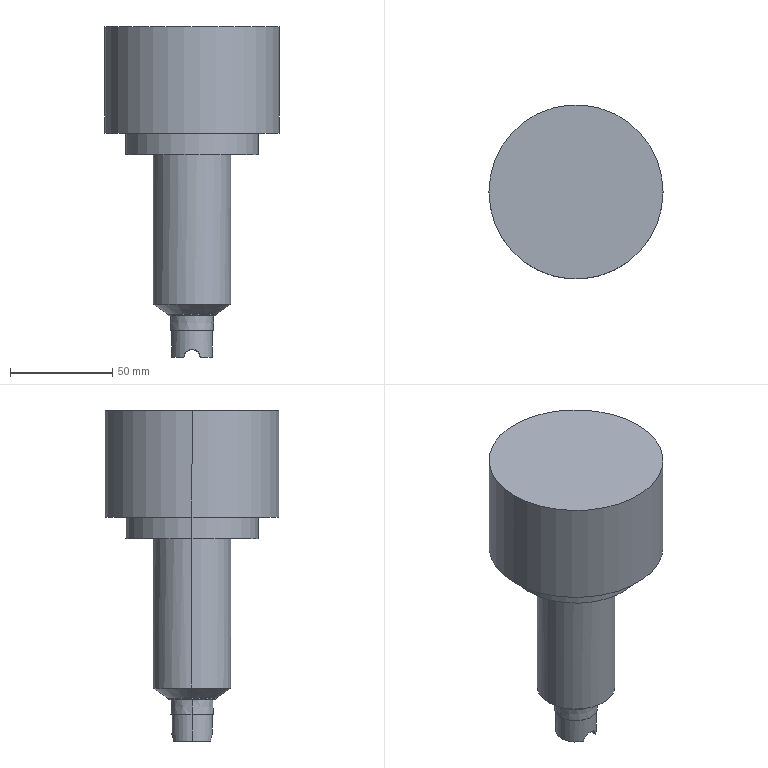Part | STEP file | 4-20.sldasm-Part-424 | 1 solid | 25 faces | box 85 x 85 x 161.455 mm | volume 422772 mm3 | cylinder 10 | plane 7 | cone 6 | spline 2 | commonest cylinder face diameters 19.999 x2 24 x2 38 x2 65 x2 85 x2